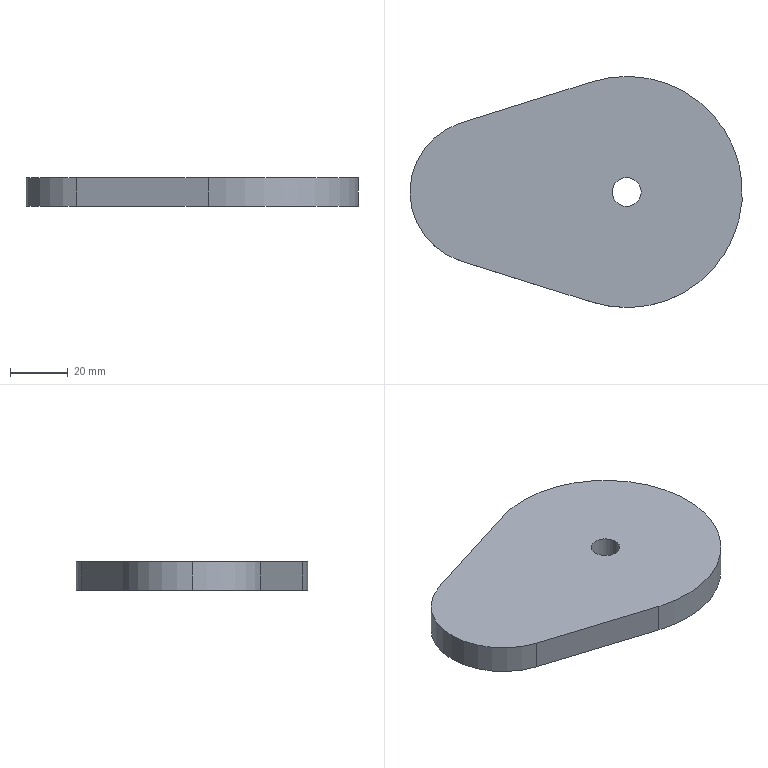Part | SolidWorks | features Extrusion 1 | 1 solid | 9 faces | box 115 x 80 x 10 mm | volume 68139 mm3 | cylinder 5 | plane 4 | commonest cylinder face diameters 10 x2 50 x2 80 x1
STEP:
#1=CARTESIAN_POINT('',(-5.,0.,10.));
#2=VERTEX_POINT('',#1);
#3=CARTESIAN_POINT('',(5.,0.,10.));
#4=VERTEX_POINT('',#3);
#5=CARTESIAN_POINT('',(0.,0.,10.));
#6=DIRECTION('',(0.,0.,1.));
#7=DIRECTION('',(1.,0.,0.));
#8=AXIS2_PLACEMENT_3D('',#5,#6,#7);
#9=CIRCLE('',#8,5.);
#10=EDGE_CURVE('',#2,#4,#9,.T.);
#11=ORIENTED_EDGE('',*,*,#10,.T.);
#12=CARTESIAN_POINT('',(5.,0.,0.));
#13=VERTEX_POINT('',#12);
#14=CARTESIAN_POINT('',(5.,0.,10.));
#15=DIRECTION('',(0.,0.,-1.));
#16=VECTOR('',#15,1000.);
#17=LINE('',#14,#16);
#18=EDGE_CURVE('',#4,#13,#17,.T.);
#19=ORIENTED_EDGE('',*,*,#18,.T.);
#20=CARTESIAN_POINT('',(-5.,0.,0.));
#21=VERTEX_POINT('',#20);
#22=CARTESIAN_POINT('',(0.,0.,0.));
#23=DIRECTION('',(0.,0.,1.));
#24=DIRECTION('',(1.,0.,0.));
#25=AXIS2_PLACEMENT_3D('',#22,#23,#24);
#26=CIRCLE('',#25,5.);
#27=EDGE_CURVE('',#21,#13,#26,.T.);
#28=ORIENTED_EDGE('',*,*,#27,.F.);
#29=CARTESIAN_POINT('',(-5.,0.,10.));
#30=DIRECTION('',(0.,0.,-1.));
#31=VECTOR('',#30,1000.);
#32=LINE('',#29,#31);
#33=EDGE_CURVE('',#2,#21,#32,.T.);
#34=ORIENTED_EDGE('',*,*,#33,.F.);
#35=EDGE_LOOP('',(#11,#19,#28,#34));
#36=FACE_OUTER_BOUND('',#35,.T.);
#37=CARTESIAN_POINT('',(0.,0.,10.));
#38=DIRECTION('',(0.,0.,-1.));
#39=DIRECTION('',(-1.,0.,0.));
#40=AXIS2_PLACEMENT_3D('',#37,#38,#39);
#41=CYLINDRICAL_SURFACE('',#40,5.);
#42=ADVANCED_FACE('',(#36),#41,.F.);
#43=CARTESIAN_POINT('',(-75.,0.,10.));
#44=VERTEX_POINT('',#43);
#45=CARTESIAN_POINT('',(-57.5,-23.848,10.));
#46=VERTEX_POINT('',#45);
#47=CARTESIAN_POINT('',(-50.,0.,10.));
#48=DIRECTION('',(0.,0.,1.));
#49=DIRECTION('',(1.,0.,0.));
#50=AXIS2_PLACEMENT_3D('',#47,#48,#49);
#51=CIRCLE('',#50,25.);
#52=EDGE_CURVE('',#44,#46,#51,.T.);
#53=ORIENTED_EDGE('',*,*,#52,.F.);
#54=CARTESIAN_POINT('',(-75.,0.,0.));
#55=VERTEX_POINT('',#54);
#56=CARTESIAN_POINT('',(-75.,0.,10.));
#57=DIRECTION('',(0.,0.,-1.));
#58=VECTOR('',#57,1000.);
#59=LINE('',#56,#58);
#60=EDGE_CURVE('',#44,#55,#59,.T.);
#61=ORIENTED_EDGE('',*,*,#60,.T.);
#62=CARTESIAN_POINT('',(-57.5,-23.848,0.));
#63=VERTEX_POINT('',#62);
#64=CARTESIAN_POINT('',(-50.,0.,0.));
#65=DIRECTION('',(0.,0.,1.));
#66=DIRECTION('',(1.,0.,0.));
#67=AXIS2_PLACEMENT_3D('',#64,#65,#66);
#68=CIRCLE('',#67,25.);
#69=EDGE_CURVE('',#55,#63,#68,.T.);
#70=ORIENTED_EDGE('',*,*,#69,.T.);
#71=CARTESIAN_POINT('',(-57.5,-23.848,10.));
#72=DIRECTION('',(0.,0.,-1.));
#73=VECTOR('',#72,1000.);
#74=LINE('',#71,#73);
#75=EDGE_CURVE('',#46,#63,#74,.T.);
#76=ORIENTED_EDGE('',*,*,#75,.F.);
#77=EDGE_LOOP('',(#53,#61,#70,#76));
#78=FACE_OUTER_BOUND('',#77,.T.);
#79=CARTESIAN_POINT('',(-50.,0.,10.));
#80=DIRECTION('',(0.,0.,-1.));
#81=DIRECTION('',(-1.,0.,0.));
#82=AXIS2_PLACEMENT_3D('',#79,#80,#81);
#83=CYLINDRICAL_SURFACE('',#82,25.);
#84=ADVANCED_FACE('',(#78),#83,.T.);
#85=CARTESIAN_POINT('',(-57.5,23.848,10.));
#86=VERTEX_POINT('',#85);
#87=CARTESIAN_POINT('',(-50.,0.,10.));
#88=DIRECTION('',(0.,0.,1.));
#89=DIRECTION('',(1.,0.,0.));
#90=AXIS2_PLACEMENT_3D('',#87,#88,#89);
#91=CIRCLE('',#90,25.);
#92=EDGE_CURVE('',#86,#44,#91,.T.);
#93=ORIENTED_EDGE('',*,*,#92,.T.);
#94=ORIENTED_EDGE('',*,*,#52,.T.);
#95=CARTESIAN_POINT('',(-12.,-38.158,10.));
#96=VERTEX_POINT('',#95);
#97=CARTESIAN_POINT('',(-57.5,-23.848,10.));
#98=DIRECTION('',(0.9539,-0.3,0.));
#99=VECTOR('',#98,1000.);
#100=LINE('',#97,#99);
#101=EDGE_CURVE('',#46,#96,#100,.T.);
#102=ORIENTED_EDGE('',*,*,#101,.T.);
#103=CARTESIAN_POINT('',(-12.,38.158,10.));
#104=VERTEX_POINT('',#103);
#105=CARTESIAN_POINT('',(0.,0.,10.));
#106=DIRECTION('',(0.,0.,1.));
#107=DIRECTION('',(1.,0.,0.));
#108=AXIS2_PLACEMENT_3D('',#105,#106,#107);
#109=CIRCLE('',#108,40.);
#110=EDGE_CURVE('',#96,#104,#109,.T.);
#111=ORIENTED_EDGE('',*,*,#110,.T.);
#112=CARTESIAN_POINT('',(-57.5,23.848,10.));
#113=DIRECTION('',(-0.9539,-0.3,0.));
#114=VECTOR('',#113,1000.);
#115=LINE('',#112,#114);
#116=EDGE_CURVE('',#104,#86,#115,.T.);
#117=ORIENTED_EDGE('',*,*,#116,.T.);
#118=EDGE_LOOP('',(#93,#94,#102,#111,#117));
#119=FACE_OUTER_BOUND('',#118,.T.);
#120=ORIENTED_EDGE('',*,*,#10,.F.);
#121=CARTESIAN_POINT('',(0.,0.,10.));
#122=DIRECTION('',(0.,0.,1.));
#123=DIRECTION('',(1.,0.,0.));
#124=AXIS2_PLACEMENT_3D('',#121,#122,#123);
#125=CIRCLE('',#124,5.);
#126=EDGE_CURVE('',#4,#2,#125,.T.);
#127=ORIENTED_EDGE('',*,*,#126,.F.);
#128=EDGE_LOOP('',(#120,#127));
#129=FACE_BOUND('',#128,.T.);
#130=CARTESIAN_POINT('',(-50.,0.,10.));
#131=DIRECTION('',(0.,0.,1.));
#132=DIRECTION('',(1.,0.,0.));
#133=AXIS2_PLACEMENT_3D('',#130,#131,#132);
#134=PLANE('',#133);
#135=ADVANCED_FACE('',(#119,#129),#134,.T.);
#136=CARTESIAN_POINT('',(-57.5,23.848,0.));
#137=VERTEX_POINT('',#136);
#138=CARTESIAN_POINT('',(-50.,0.,0.));
#139=DIRECTION('',(0.,0.,1.));
#140=DIRECTION('',(1.,0.,0.));
#141=AXIS2_PLACEMENT_3D('',#138,#139,#140);
#142=CIRCLE('',#141,25.);
#143=EDGE_CURVE('',#137,#55,#142,.T.);
#144=ORIENTED_EDGE('',*,*,#143,.F.);
#145=CARTESIAN_POINT('',(-12.,38.158,0.));
#146=VERTEX_POINT('',#145);
#147=CARTESIAN_POINT('',(-57.5,23.848,0.));
#148=DIRECTION('',(-0.9539,-0.3,0.));
#149=VECTOR('',#148,1000.);
#150=LINE('',#147,#149);
#151=EDGE_CURVE('',#146,#137,#150,.T.);
#152=ORIENTED_EDGE('',*,*,#151,.F.);
#153=CARTESIAN_POINT('',(-12.,-38.158,0.));
#154=VERTEX_POINT('',#153);
#155=CARTESIAN_POINT('',(0.,0.,0.));
#156=DIRECTION('',(0.,0.,1.));
#157=DIRECTION('',(1.,0.,0.));
#158=AXIS2_PLACEMENT_3D('',#155,#156,#157);
#159=CIRCLE('',#158,40.);
#160=EDGE_CURVE('',#154,#146,#159,.T.);
#161=ORIENTED_EDGE('',*,*,#160,.F.);
#162=CARTESIAN_POINT('',(-57.5,-23.848,0.));
#163=DIRECTION('',(0.9539,-0.3,0.));
#164=VECTOR('',#163,1000.);
#165=LINE('',#162,#164);
#166=EDGE_CURVE('',#63,#154,#165,.T.);
#167=ORIENTED_EDGE('',*,*,#166,.F.);
#168=ORIENTED_EDGE('',*,*,#69,.F.);
#169=EDGE_LOOP('',(#144,#152,#161,#167,#168));
#170=FACE_OUTER_BOUND('',#169,.T.);
#171=ORIENTED_EDGE('',*,*,#27,.T.);
#172=CARTESIAN_POINT('',(0.,0.,0.));
#173=DIRECTION('',(0.,0.,1.));
#174=DIRECTION('',(1.,0.,0.));
#175=AXIS2_PLACEMENT_3D('',#172,#173,#174);
#176=CIRCLE('',#175,5.);
#177=EDGE_CURVE('',#13,#21,#176,.T.);
#178=ORIENTED_EDGE('',*,*,#177,.T.);
#179=EDGE_LOOP('',(#171,#178));
#180=FACE_BOUND('',#179,.T.);
#181=CARTESIAN_POINT('',(-50.,0.,0.));
#182=DIRECTION('',(0.,0.,1.));
#183=DIRECTION('',(1.,0.,0.));
#184=AXIS2_PLACEMENT_3D('',#181,#182,#183);
#185=PLANE('',#184);
#186=ADVANCED_FACE('',(#170,#180),#185,.F.);
#187=ORIENTED_EDGE('',*,*,#60,.F.);
#188=ORIENTED_EDGE('',*,*,#92,.F.);
#189=CARTESIAN_POINT('',(-57.5,23.848,10.));
#190=DIRECTION('',(0.,0.,-1.));
#191=VECTOR('',#190,1000.);
#192=LINE('',#189,#191);
#193=EDGE_CURVE('',#86,#137,#192,.T.);
#194=ORIENTED_EDGE('',*,*,#193,.T.);
#195=ORIENTED_EDGE('',*,*,#143,.T.);
#196=EDGE_LOOP('',(#187,#188,#194,#195));
#197=FACE_OUTER_BOUND('',#196,.T.);
#198=CARTESIAN_POINT('',(-50.,0.,10.));
#199=DIRECTION('',(0.,0.,-1.));
#200=DIRECTION('',(-1.,0.,0.));
#201=AXIS2_PLACEMENT_3D('',#198,#199,#200);
#202=CYLINDRICAL_SURFACE('',#201,25.);
#203=ADVANCED_FACE('',(#197),#202,.T.);
#204=ORIENTED_EDGE('',*,*,#166,.T.);
#205=CARTESIAN_POINT('',(-12.,-38.158,10.));
#206=DIRECTION('',(0.,0.,-1.));
#207=VECTOR('',#206,1000.);
#208=LINE('',#205,#207);
#209=EDGE_CURVE('',#96,#154,#208,.T.);
#210=ORIENTED_EDGE('',*,*,#209,.F.);
#211=ORIENTED_EDGE('',*,*,#101,.F.);
#212=ORIENTED_EDGE('',*,*,#75,.T.);
#213=EDGE_LOOP('',(#204,#210,#211,#212));
#214=FACE_OUTER_BOUND('',#213,.T.);
#215=CARTESIAN_POINT('',(-57.5,-23.848,10.));
#216=DIRECTION('',(0.3,0.9539,0.));
#217=DIRECTION('',(-0.9539,0.3,0.));
#218=AXIS2_PLACEMENT_3D('',#215,#216,#217);
#219=PLANE('',#218);
#220=ADVANCED_FACE('',(#214),#219,.F.);
#221=ORIENTED_EDGE('',*,*,#160,.T.);
#222=CARTESIAN_POINT('',(-12.,38.158,10.));
#223=DIRECTION('',(0.,0.,-1.));
#224=VECTOR('',#223,1000.);
#225=LINE('',#222,#224);
#226=EDGE_CURVE('',#104,#146,#225,.T.);
#227=ORIENTED_EDGE('',*,*,#226,.F.);
#228=ORIENTED_EDGE('',*,*,#110,.F.);
#229=ORIENTED_EDGE('',*,*,#209,.T.);
#230=EDGE_LOOP('',(#221,#227,#228,#229));
#231=FACE_OUTER_BOUND('',#230,.T.);
#232=CARTESIAN_POINT('',(0.,0.,10.));
#233=DIRECTION('',(0.,0.,-1.));
#234=DIRECTION('',(-1.,0.,0.));
#235=AXIS2_PLACEMENT_3D('',#232,#233,#234);
#236=CYLINDRICAL_SURFACE('',#235,40.);
#237=ADVANCED_FACE('',(#231),#236,.T.);
#238=ORIENTED_EDGE('',*,*,#151,.T.);
#239=ORIENTED_EDGE('',*,*,#193,.F.);
#240=ORIENTED_EDGE('',*,*,#116,.F.);
#241=ORIENTED_EDGE('',*,*,#226,.T.);
#242=EDGE_LOOP('',(#238,#239,#240,#241));
#243=FACE_OUTER_BOUND('',#242,.T.);
#244=CARTESIAN_POINT('',(-57.5,23.848,10.));
#245=DIRECTION('',(0.3,-0.9539,0.));
#246=DIRECTION('',(0.9539,0.3,0.));
#247=AXIS2_PLACEMENT_3D('',#244,#245,#246);
#248=PLANE('',#247);
#249=ADVANCED_FACE('',(#243),#248,.F.);
#250=ORIENTED_EDGE('',*,*,#18,.F.);
#251=ORIENTED_EDGE('',*,*,#126,.T.);
#252=ORIENTED_EDGE('',*,*,#33,.T.);
#253=ORIENTED_EDGE('',*,*,#177,.F.);
#254=EDGE_LOOP('',(#250,#251,#252,#253));
#255=FACE_OUTER_BOUND('',#254,.T.);
#256=CARTESIAN_POINT('',(0.,0.,10.));
#257=DIRECTION('',(0.,0.,-1.));
#258=DIRECTION('',(-1.,0.,0.));
#259=AXIS2_PLACEMENT_3D('',#256,#257,#258);
#260=CYLINDRICAL_SURFACE('',#259,5.);
#261=ADVANCED_FACE('',(#255),#260,.F.);
#262=CLOSED_SHELL('',(#42,#84,#135,#186,#203,#220,#237,#249,#261));
#263=MANIFOLD_SOLID_BREP('',#262);
#264=CARTESIAN_POINT('',(0.,0.,0.));
#265=DIRECTION('',(0.,0.,1.));
#266=DIRECTION('',(1.,0.,0.));
#267=AXIS2_PLACEMENT_3D('',#264,#265,#266);
#268=(LENGTH_UNIT()NAMED_UNIT(*)SI_UNIT(.MILLI.,.METRE.));
#269=UNCERTAINTY_MEASURE_WITH_UNIT(LENGTH_MEASURE(0.00001),#268,'','');
#270=(NAMED_UNIT(*)PLANE_ANGLE_UNIT()SI_UNIT($,.RADIAN.));
#271=(NAMED_UNIT(*)SI_UNIT($,.STERADIAN.)SOLID_ANGLE_UNIT());
#272=(GEOMETRIC_REPRESENTATION_CONTEXT(3)GLOBAL_UNCERTAINTY_ASSIGNED_CONTEXT((#269))GLOBAL_UNIT_ASSIGNED_CONTEXT((#268,#270,#271))REPRESENTATION_CONTEXT('',''));
#273=ADVANCED_BREP_SHAPE_REPRESENTATION('',(#263,#267),#272);